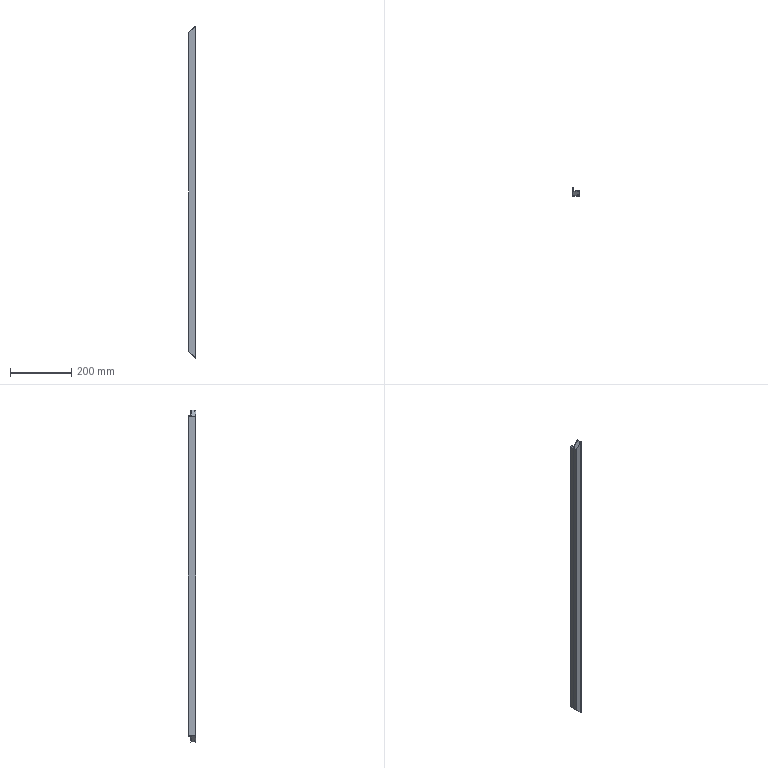Part | SolidWorks | features ICE 2, Extrusion 1 | 1 solid | 39 faces | box 22 x 25 x 1081 mm | volume 350449 mm3 | plane 22 | cylinder 17 | commonest cylinder face diameters 0.6 x2 2 x2 3.8 x2 23.6 x2 26 x2 0.97 x1
STEP:
#1=CARTESIAN_POINT('',(27.064,65.097,1061.634));
#2=VERTEX_POINT('',#1);
#3=CARTESIAN_POINT('',(26.938,66.899,1061.509));
#4=VERTEX_POINT('',#3);
#5=CARTESIAN_POINT('',(27.064,65.097,1061.634));
#6=CARTESIAN_POINT('',(26.98,65.694,1061.55));
#7=CARTESIAN_POINT('',(26.938,66.296,1061.509));
#8=CARTESIAN_POINT('',(26.938,66.899,1061.509));
#9=(BOUNDED_CURVE()B_SPLINE_CURVE(3,(#5,#6,#7,#8),.UNSPECIFIED.,.F.,.F.)B_SPLINE_CURVE_WITH_KNOTS((4,4),(6.144,6.283),.UNSPECIFIED.)CURVE()GEOMETRIC_REPRESENTATION_ITEM()RATIONAL_B_SPLINE_CURVE((1.,0.9984,0.9984,1.))REPRESENTATION_ITEM(''));
#10=EDGE_CURVE('',#2,#4,#9,.T.);
#11=ORIENTED_EDGE('',*,*,#10,.T.);
#12=CARTESIAN_POINT('',(26.938,66.899,19.491));
#13=VERTEX_POINT('',#12);
#14=CARTESIAN_POINT('',(26.938,66.899,1081.));
#15=DIRECTION('',(0.,0.,-1.));
#16=VECTOR('',#15,1000.);
#17=LINE('',#14,#16);
#18=EDGE_CURVE('',#4,#13,#17,.T.);
#19=ORIENTED_EDGE('',*,*,#18,.T.);
#20=CARTESIAN_POINT('',(27.064,65.097,19.366));
#21=VERTEX_POINT('',#20);
#22=CARTESIAN_POINT('',(27.064,65.097,19.366));
#23=CARTESIAN_POINT('',(26.98,65.694,19.45));
#24=CARTESIAN_POINT('',(26.938,66.296,19.491));
#25=CARTESIAN_POINT('',(26.938,66.899,19.491));
#26=(BOUNDED_CURVE()B_SPLINE_CURVE(3,(#22,#23,#24,#25),.UNSPECIFIED.,.F.,.T.)B_SPLINE_CURVE_WITH_KNOTS((4,4),(3.002,3.142),.UNSPECIFIED.)CURVE()GEOMETRIC_REPRESENTATION_ITEM()RATIONAL_B_SPLINE_CURVE((1.,0.9984,0.9984,1.))REPRESENTATION_ITEM(''));
#27=EDGE_CURVE('',#21,#13,#26,.T.);
#28=ORIENTED_EDGE('',*,*,#27,.F.);
#29=CARTESIAN_POINT('',(27.064,65.097,1081.));
#30=DIRECTION('',(0.,0.,-1.));
#31=VECTOR('',#30,1000.);
#32=LINE('',#29,#31);
#33=EDGE_CURVE('',#2,#21,#32,.T.);
#34=ORIENTED_EDGE('',*,*,#33,.F.);
#35=EDGE_LOOP('',(#11,#19,#28,#34));
#36=FACE_OUTER_BOUND('',#35,.T.);
#37=CARTESIAN_POINT('',(39.938,66.899,1081.));
#38=DIRECTION('',(0.,0.,-1.));
#39=DIRECTION('',(-1.,0.,0.));
#40=AXIS2_PLACEMENT_3D('',#37,#38,#39);
#41=CYLINDRICAL_SURFACE('',#40,13.);
#42=ADVANCED_FACE('',(#36),#41,.T.);
#43=CARTESIAN_POINT('',(28.252,68.536,1062.823));
#44=VERTEX_POINT('',#43);
#45=CARTESIAN_POINT('',(28.138,66.899,1062.709));
#46=VERTEX_POINT('',#45);
#47=CARTESIAN_POINT('',(28.252,68.536,1062.823));
#48=CARTESIAN_POINT('',(28.176,67.993,1062.747));
#49=CARTESIAN_POINT('',(28.138,67.447,1062.709));
#50=CARTESIAN_POINT('',(28.138,66.899,1062.709));
#51=(BOUNDED_CURVE()B_SPLINE_CURVE(3,(#47,#48,#49,#50),.UNSPECIFIED.,.F.,.F.)B_SPLINE_CURVE_WITH_KNOTS((4,4),(6.144,6.283),.UNSPECIFIED.)CURVE()GEOMETRIC_REPRESENTATION_ITEM()RATIONAL_B_SPLINE_CURVE((1.,0.9984,0.9984,1.))REPRESENTATION_ITEM(''));
#52=EDGE_CURVE('',#44,#46,#51,.T.);
#53=ORIENTED_EDGE('',*,*,#52,.T.);
#54=CARTESIAN_POINT('',(28.138,66.899,18.291));
#55=VERTEX_POINT('',#54);
#56=CARTESIAN_POINT('',(28.138,66.899,1081.));
#57=DIRECTION('',(0.,0.,-1.));
#58=VECTOR('',#57,1000.);
#59=LINE('',#56,#58);
#60=EDGE_CURVE('',#46,#55,#59,.T.);
#61=ORIENTED_EDGE('',*,*,#60,.T.);
#62=CARTESIAN_POINT('',(28.252,68.536,18.177));
#63=VERTEX_POINT('',#62);
#64=CARTESIAN_POINT('',(28.252,68.536,18.177));
#65=CARTESIAN_POINT('',(28.176,67.993,18.253));
#66=CARTESIAN_POINT('',(28.138,67.447,18.291));
#67=CARTESIAN_POINT('',(28.138,66.899,18.291));
#68=(BOUNDED_CURVE()B_SPLINE_CURVE(3,(#64,#65,#66,#67),.UNSPECIFIED.,.F.,.F.)B_SPLINE_CURVE_WITH_KNOTS((4,4),(3.002,3.142),.UNSPECIFIED.)CURVE()GEOMETRIC_REPRESENTATION_ITEM()RATIONAL_B_SPLINE_CURVE((1.,0.9984,0.9984,1.))REPRESENTATION_ITEM(''));
#69=EDGE_CURVE('',#63,#55,#68,.T.);
#70=ORIENTED_EDGE('',*,*,#69,.F.);
#71=CARTESIAN_POINT('',(28.252,68.536,1081.));
#72=DIRECTION('',(0.,0.,-1.));
#73=VECTOR('',#72,1000.);
#74=LINE('',#71,#73);
#75=EDGE_CURVE('',#44,#63,#74,.T.);
#76=ORIENTED_EDGE('',*,*,#75,.F.);
#77=EDGE_LOOP('',(#53,#61,#70,#76));
#78=FACE_OUTER_BOUND('',#77,.T.);
#79=CARTESIAN_POINT('',(39.938,66.899,1081.));
#80=DIRECTION('',(0.,0.,-1.));
#81=DIRECTION('',(-1.,0.,0.));
#82=AXIS2_PLACEMENT_3D('',#79,#80,#81);
#83=CYLINDRICAL_SURFACE('',#82,11.8);
#84=ADVANCED_FACE('',(#78),#83,.F.);
#85=CARTESIAN_POINT('',(44.608,52.847,1079.178));
#86=VERTEX_POINT('',#85);
#87=CARTESIAN_POINT('',(41.6,51.304,1076.17));
#88=VERTEX_POINT('',#87);
#89=CARTESIAN_POINT('',(44.608,52.847,1079.178));
#90=CARTESIAN_POINT('',(43.172,53.878,1077.743));
#91=CARTESIAN_POINT('',(41.6,53.071,1076.17));
#92=CARTESIAN_POINT('',(41.6,51.304,1076.17));
#93=(BOUNDED_CURVE()B_SPLINE_CURVE(3,(#89,#90,#91,#92),.UNSPECIFIED.,.F.,.F.)B_SPLINE_CURVE_WITH_KNOTS((4,4),(4.09,6.283),.UNSPECIFIED.)CURVE()GEOMETRIC_REPRESENTATION_ITEM()RATIONAL_B_SPLINE_CURVE((1.,0.6376,0.6376,1.))REPRESENTATION_ITEM(''));
#94=EDGE_CURVE('',#86,#88,#93,.T.);
#95=ORIENTED_EDGE('',*,*,#94,.T.);
#96=CARTESIAN_POINT('',(41.6,51.304,4.83));
#97=VERTEX_POINT('',#96);
#98=CARTESIAN_POINT('',(41.6,51.304,1081.));
#99=DIRECTION('',(0.,0.,-1.));
#100=VECTOR('',#99,1000.);
#101=LINE('',#98,#100);
#102=EDGE_CURVE('',#88,#97,#101,.T.);
#103=ORIENTED_EDGE('',*,*,#102,.T.);
#104=CARTESIAN_POINT('',(44.608,52.847,1.822));
#105=VERTEX_POINT('',#104);
#106=CARTESIAN_POINT('',(44.608,52.847,1.822));
#107=CARTESIAN_POINT('',(43.172,53.878,3.257));
#108=CARTESIAN_POINT('',(41.6,53.071,4.83));
#109=CARTESIAN_POINT('',(41.6,51.304,4.83));
#110=(BOUNDED_CURVE()B_SPLINE_CURVE(3,(#106,#107,#108,#109),.UNSPECIFIED.,.F.,.F.)B_SPLINE_CURVE_WITH_KNOTS((4,4),(0.948,3.142),.UNSPECIFIED.)CURVE()GEOMETRIC_REPRESENTATION_ITEM()RATIONAL_B_SPLINE_CURVE((1.,0.6376,0.6376,1.))REPRESENTATION_ITEM(''));
#111=EDGE_CURVE('',#105,#97,#110,.T.);
#112=ORIENTED_EDGE('',*,*,#111,.F.);
#113=CARTESIAN_POINT('',(44.608,52.847,1081.));
#114=DIRECTION('',(0.,0.,-1.));
#115=VECTOR('',#114,1000.);
#116=LINE('',#113,#115);
#117=EDGE_CURVE('',#86,#105,#116,.T.);
#118=ORIENTED_EDGE('',*,*,#117,.F.);
#119=EDGE_LOOP('',(#95,#103,#112,#118));
#120=FACE_OUTER_BOUND('',#119,.T.);
#121=CARTESIAN_POINT('',(43.5,51.304,1081.));
#122=DIRECTION('',(0.,0.,-1.));
#123=DIRECTION('',(-1.,0.,0.));
#124=AXIS2_PLACEMENT_3D('',#121,#122,#123);
#125=CYLINDRICAL_SURFACE('',#124,1.9);
#126=ADVANCED_FACE('',(#120),#125,.F.);
#127=CARTESIAN_POINT('',(45.44,49.348,1080.01));
#128=VERTEX_POINT('',#127);
#129=CARTESIAN_POINT('',(45.43,49.204,1080.));
#130=VERTEX_POINT('',#129);
#131=CARTESIAN_POINT('',(45.44,49.348,1080.01));
#132=CARTESIAN_POINT('',(45.433,49.3,1080.003));
#133=CARTESIAN_POINT('',(45.43,49.252,1080.));
#134=CARTESIAN_POINT('',(45.43,49.204,1080.));
#135=(BOUNDED_CURVE()B_SPLINE_CURVE(3,(#131,#132,#133,#134),.UNSPECIFIED.,.F.,.F.)B_SPLINE_CURVE_WITH_KNOTS((4,4),(6.138,6.283),.UNSPECIFIED.)CURVE()GEOMETRIC_REPRESENTATION_ITEM()RATIONAL_B_SPLINE_CURVE((1.,0.9983,0.9983,1.))REPRESENTATION_ITEM(''));
#136=EDGE_CURVE('',#128,#130,#135,.T.);
#137=ORIENTED_EDGE('',*,*,#136,.T.);
#138=CARTESIAN_POINT('',(45.43,49.204,1.));
#139=VERTEX_POINT('',#138);
#140=CARTESIAN_POINT('',(45.43,49.204,1081.));
#141=DIRECTION('',(0.,0.,-1.));
#142=VECTOR('',#141,1000.);
#143=LINE('',#140,#142);
#144=EDGE_CURVE('',#130,#139,#143,.T.);
#145=ORIENTED_EDGE('',*,*,#144,.T.);
#146=CARTESIAN_POINT('',(45.44,49.348,0.9896));
#147=VERTEX_POINT('',#146);
#148=CARTESIAN_POINT('',(45.44,49.348,0.9896));
#149=CARTESIAN_POINT('',(45.433,49.3,0.9965));
#150=CARTESIAN_POINT('',(45.43,49.252,1.));
#151=CARTESIAN_POINT('',(45.43,49.204,1.));
#152=(BOUNDED_CURVE()B_SPLINE_CURVE(3,(#148,#149,#150,#151),.UNSPECIFIED.,.F.,.F.)B_SPLINE_CURVE_WITH_KNOTS((4,4),(2.997,3.142),.UNSPECIFIED.)CURVE()GEOMETRIC_REPRESENTATION_ITEM()RATIONAL_B_SPLINE_CURVE((1.,0.9983,0.9983,1.))REPRESENTATION_ITEM(''));
#153=EDGE_CURVE('',#147,#139,#152,.T.);
#154=ORIENTED_EDGE('',*,*,#153,.F.);
#155=CARTESIAN_POINT('',(45.44,49.348,1081.));
#156=DIRECTION('',(0.,0.,-1.));
#157=VECTOR('',#156,1000.);
#158=LINE('',#155,#157);
#159=EDGE_CURVE('',#128,#147,#158,.T.);
#160=ORIENTED_EDGE('',*,*,#159,.F.);
#161=EDGE_LOOP('',(#137,#145,#154,#160));
#162=FACE_OUTER_BOUND('',#161,.T.);
#163=CARTESIAN_POINT('',(46.43,49.204,1081.));
#164=DIRECTION('',(0.,0.,-1.));
#165=DIRECTION('',(-1.,0.,0.));
#166=AXIS2_PLACEMENT_3D('',#163,#164,#165);
#167=CYLINDRICAL_SURFACE('',#166,1.);
#168=ADVANCED_FACE('',(#162),#167,.F.);
#169=CARTESIAN_POINT('',(24.43,48.204,1059.));
#170=VERTEX_POINT('',#169);
#171=CARTESIAN_POINT('',(24.43,48.204,22.));
#172=VERTEX_POINT('',#171);
#173=CARTESIAN_POINT('',(24.43,48.204,1081.));
#174=DIRECTION('',(0.,0.,-1.));
#175=VECTOR('',#174,1000.);
#176=LINE('',#173,#175);
#177=EDGE_CURVE('',#170,#172,#176,.T.);
#178=ORIENTED_EDGE('',*,*,#177,.F.);
#179=CARTESIAN_POINT('',(24.43,73.204,1059.));
#180=VERTEX_POINT('',#179);
#181=CARTESIAN_POINT('',(24.43,78.204,1059.));
#182=DIRECTION('',(0.,-1.,0.));
#183=VECTOR('',#182,1000.);
#184=LINE('',#181,#183);
#185=EDGE_CURVE('',#180,#170,#184,.T.);
#186=ORIENTED_EDGE('',*,*,#185,.F.);
#187=CARTESIAN_POINT('',(24.43,73.204,22.));
#188=VERTEX_POINT('',#187);
#189=CARTESIAN_POINT('',(24.43,73.204,1081.));
#190=DIRECTION('',(0.,0.,-1.));
#191=VECTOR('',#190,1000.);
#192=LINE('',#189,#191);
#193=EDGE_CURVE('',#180,#188,#192,.T.);
#194=ORIENTED_EDGE('',*,*,#193,.T.);
#195=CARTESIAN_POINT('',(24.43,-1303.688,22.));
#196=DIRECTION('',(0.,1.,0.));
#197=VECTOR('',#196,1000.);
#198=LINE('',#195,#197);
#199=EDGE_CURVE('',#172,#188,#198,.T.);
#200=ORIENTED_EDGE('',*,*,#199,.F.);
#201=EDGE_LOOP('',(#178,#186,#194,#200));
#202=FACE_OUTER_BOUND('',#201,.T.);
#203=CARTESIAN_POINT('',(24.43,48.204,1081.));
#204=DIRECTION('',(1.,0.,0.));
#205=DIRECTION('',(0.,0.,-1.));
#206=AXIS2_PLACEMENT_3D('',#203,#204,#205);
#207=PLANE('',#206);
#208=ADVANCED_FACE('',(#202),#207,.F.);
#209=CARTESIAN_POINT('',(46.43,48.204,1081.));
#210=VERTEX_POINT('',#209);
#211=CARTESIAN_POINT('',(46.43,48.204,0.));
#212=VERTEX_POINT('',#211);
#213=CARTESIAN_POINT('',(46.43,48.204,1081.));
#214=DIRECTION('',(0.,0.,-1.));
#215=VECTOR('',#214,1000.);
#216=LINE('',#213,#215);
#217=EDGE_CURVE('',#210,#212,#216,.T.);
#218=ORIENTED_EDGE('',*,*,#217,.F.);
#219=CARTESIAN_POINT('',(46.43,48.204,1081.));
#220=DIRECTION('',(0.7071,0.,0.7071));
#221=VECTOR('',#220,1000.);
#222=LINE('',#219,#221);
#223=EDGE_CURVE('',#170,#210,#222,.T.);
#224=ORIENTED_EDGE('',*,*,#223,.F.);
#225=ORIENTED_EDGE('',*,*,#177,.T.);
#226=CARTESIAN_POINT('',(-505.07,48.204,551.5));
#227=DIRECTION('',(-0.7071,0.,0.7071));
#228=VECTOR('',#227,1000.);
#229=LINE('',#226,#228);
#230=EDGE_CURVE('',#212,#172,#229,.T.);
#231=ORIENTED_EDGE('',*,*,#230,.F.);
#232=EDGE_LOOP('',(#218,#224,#225,#231));
#233=FACE_OUTER_BOUND('',#232,.T.);
#234=CARTESIAN_POINT('',(24.43,48.204,1081.));
#235=DIRECTION('',(0.,1.,0.));
#236=DIRECTION('',(0.,0.,1.));
#237=AXIS2_PLACEMENT_3D('',#234,#235,#236);
#238=PLANE('',#237);
#239=ADVANCED_FACE('',(#233),#238,.F.);
#240=ORIENTED_EDGE('',*,*,#144,.F.);
#241=CARTESIAN_POINT('',(45.43,49.204,1080.));
#242=CARTESIAN_POINT('',(45.43,48.618,1080.));
#243=CARTESIAN_POINT('',(45.844,48.204,1080.414));
#244=CARTESIAN_POINT('',(46.43,48.204,1081.));
#245=(BOUNDED_CURVE()B_SPLINE_CURVE(3,(#241,#242,#243,#244),.UNSPECIFIED.,.F.,.F.)B_SPLINE_CURVE_WITH_KNOTS((4,4),(0.,1.571),.UNSPECIFIED.)CURVE()GEOMETRIC_REPRESENTATION_ITEM()RATIONAL_B_SPLINE_CURVE((1.,0.8047,0.8047,1.))REPRESENTATION_ITEM(''));
#246=EDGE_CURVE('',#130,#210,#245,.T.);
#247=ORIENTED_EDGE('',*,*,#246,.T.);
#248=ORIENTED_EDGE('',*,*,#217,.T.);
#249=CARTESIAN_POINT('',(45.43,49.204,1.));
#250=CARTESIAN_POINT('',(45.43,48.618,1.));
#251=CARTESIAN_POINT('',(45.844,48.204,0.5858));
#252=CARTESIAN_POINT('',(46.43,48.204,0.));
#253=(BOUNDED_CURVE()B_SPLINE_CURVE(3,(#249,#250,#251,#252),.UNSPECIFIED.,.F.,.F.)B_SPLINE_CURVE_WITH_KNOTS((4,4),(3.142,4.712),.UNSPECIFIED.)CURVE()GEOMETRIC_REPRESENTATION_ITEM()RATIONAL_B_SPLINE_CURVE((1.,0.8047,0.8047,1.))REPRESENTATION_ITEM(''));
#254=EDGE_CURVE('',#139,#212,#253,.T.);
#255=ORIENTED_EDGE('',*,*,#254,.F.);
#256=EDGE_LOOP('',(#240,#247,#248,#255));
#257=FACE_OUTER_BOUND('',#256,.T.);
#258=CARTESIAN_POINT('',(46.43,49.204,1081.));
#259=DIRECTION('',(0.,0.,-1.));
#260=DIRECTION('',(-1.,0.,0.));
#261=AXIS2_PLACEMENT_3D('',#258,#259,#260);
#262=CYLINDRICAL_SURFACE('',#261,1.);
#263=ADVANCED_FACE('',(#257),#262,.F.);
#264=CARTESIAN_POINT('',(44.663,49.801,1079.233));
#265=VERTEX_POINT('',#264);
#266=CARTESIAN_POINT('',(44.663,49.801,1.767));
#267=VERTEX_POINT('',#266);
#268=CARTESIAN_POINT('',(44.663,49.801,1081.));
#269=DIRECTION('',(0.,0.,-1.));
#270=VECTOR('',#269,1000.);
#271=LINE('',#268,#270);
#272=EDGE_CURVE('',#265,#267,#271,.T.);
#273=ORIENTED_EDGE('',*,*,#272,.F.);
#274=CARTESIAN_POINT('',(44.663,49.801,1079.233));
#275=CARTESIAN_POINT('',(45.07,50.116,1079.64));
#276=CARTESIAN_POINT('',(45.514,49.857,1080.085));
#277=CARTESIAN_POINT('',(45.44,49.348,1080.01));
#278=(BOUNDED_CURVE()B_SPLINE_CURVE(3,(#274,#275,#276,#277),.UNSPECIFIED.,.F.,.F.)B_SPLINE_CURVE_WITH_KNOTS((4,4),(0.9119,3.286),.UNSPECIFIED.)CURVE()GEOMETRIC_REPRESENTATION_ITEM()RATIONAL_B_SPLINE_CURVE((1.,0.5828,0.5828,1.))REPRESENTATION_ITEM(''));
#279=EDGE_CURVE('',#265,#128,#278,.T.);
#280=ORIENTED_EDGE('',*,*,#279,.T.);
#281=ORIENTED_EDGE('',*,*,#159,.T.);
#282=CARTESIAN_POINT('',(44.663,49.801,1.767));
#283=CARTESIAN_POINT('',(45.07,50.116,1.36));
#284=CARTESIAN_POINT('',(45.514,49.857,0.9153));
#285=CARTESIAN_POINT('',(45.44,49.348,0.9896));
#286=(BOUNDED_CURVE()B_SPLINE_CURVE(3,(#282,#283,#284,#285),.UNSPECIFIED.,.F.,.F.)B_SPLINE_CURVE_WITH_KNOTS((4,4),(4.053,6.428),.UNSPECIFIED.)CURVE()GEOMETRIC_REPRESENTATION_ITEM()RATIONAL_B_SPLINE_CURVE((1.,0.5828,0.5828,1.))REPRESENTATION_ITEM(''));
#287=EDGE_CURVE('',#267,#147,#286,.T.);
#288=ORIENTED_EDGE('',*,*,#287,.F.);
#289=EDGE_LOOP('',(#273,#280,#281,#288));
#290=FACE_OUTER_BOUND('',#289,.T.);
#291=CARTESIAN_POINT('',(44.96,49.418,1081.));
#292=DIRECTION('',(0.,0.,-1.));
#293=DIRECTION('',(-1.,0.,0.));
#294=AXIS2_PLACEMENT_3D('',#291,#292,#293);
#295=CYLINDRICAL_SURFACE('',#294,0.4852);
#296=ADVANCED_FACE('',(#290),#295,.T.);
#297=ORIENTED_EDGE('',*,*,#102,.F.);
#298=CARTESIAN_POINT('',(41.6,51.304,1076.17));
#299=CARTESIAN_POINT('',(41.6,49.489,1076.17));
#300=CARTESIAN_POINT('',(43.228,48.691,1077.799));
#301=CARTESIAN_POINT('',(44.663,49.801,1079.233));
#302=(BOUNDED_CURVE()B_SPLINE_CURVE(3,(#298,#299,#300,#301),.UNSPECIFIED.,.F.,.T.)B_SPLINE_CURVE_WITH_KNOTS((4,4),(0.,2.23),.UNSPECIFIED.)CURVE()GEOMETRIC_REPRESENTATION_ITEM()RATIONAL_B_SPLINE_CURVE((1.,0.6269,0.6269,1.))REPRESENTATION_ITEM(''));
#303=EDGE_CURVE('',#88,#265,#302,.T.);
#304=ORIENTED_EDGE('',*,*,#303,.T.);
#305=ORIENTED_EDGE('',*,*,#272,.T.);
#306=CARTESIAN_POINT('',(41.6,51.304,4.83));
#307=CARTESIAN_POINT('',(41.6,49.489,4.83));
#308=CARTESIAN_POINT('',(43.228,48.691,3.201));
#309=CARTESIAN_POINT('',(44.663,49.801,1.767));
#310=(BOUNDED_CURVE()B_SPLINE_CURVE(3,(#306,#307,#308,#309),.UNSPECIFIED.,.F.,.T.)B_SPLINE_CURVE_WITH_KNOTS((4,4),(3.142,5.371),.UNSPECIFIED.)CURVE()GEOMETRIC_REPRESENTATION_ITEM()RATIONAL_B_SPLINE_CURVE((1.,0.6269,0.6269,1.))REPRESENTATION_ITEM(''));
#311=EDGE_CURVE('',#97,#267,#310,.T.);
#312=ORIENTED_EDGE('',*,*,#311,.F.);
#313=EDGE_LOOP('',(#297,#304,#305,#312));
#314=FACE_OUTER_BOUND('',#313,.T.);
#315=CARTESIAN_POINT('',(43.5,51.304,1081.));
#316=DIRECTION('',(0.,0.,-1.));
#317=DIRECTION('',(-1.,0.,0.));
#318=AXIS2_PLACEMENT_3D('',#315,#316,#317);
#319=CYLINDRICAL_SURFACE('',#318,1.9);
#320=ADVANCED_FACE('',(#314),#319,.F.);
#321=CARTESIAN_POINT('',(45.4,53.253,1079.97));
#322=VERTEX_POINT('',#321);
#323=CARTESIAN_POINT('',(45.4,53.253,1.03));
#324=VERTEX_POINT('',#323);
#325=CARTESIAN_POINT('',(45.4,53.253,1081.));
#326=DIRECTION('',(0.,0.,-1.));
#327=VECTOR('',#326,1000.);
#328=LINE('',#325,#327);
#329=EDGE_CURVE('',#322,#324,#328,.T.);
#330=ORIENTED_EDGE('',*,*,#329,.F.);
#331=CARTESIAN_POINT('',(45.4,53.253,1079.97));
#332=CARTESIAN_POINT('',(45.4,52.788,1079.97));
#333=CARTESIAN_POINT('',(44.986,52.575,1079.556));
#334=CARTESIAN_POINT('',(44.608,52.847,1079.178));
#335=(BOUNDED_CURVE()B_SPLINE_CURVE(3,(#331,#332,#333,#334),.UNSPECIFIED.,.F.,.F.)B_SPLINE_CURVE_WITH_KNOTS((4,4),(3.142,5.335),.UNSPECIFIED.)CURVE()GEOMETRIC_REPRESENTATION_ITEM()RATIONAL_B_SPLINE_CURVE((1.,0.6376,0.6376,1.))REPRESENTATION_ITEM(''));
#336=EDGE_CURVE('',#322,#86,#335,.T.);
#337=ORIENTED_EDGE('',*,*,#336,.T.);
#338=ORIENTED_EDGE('',*,*,#117,.T.);
#339=CARTESIAN_POINT('',(45.4,53.253,1.03));
#340=CARTESIAN_POINT('',(45.4,52.788,1.03));
#341=CARTESIAN_POINT('',(44.986,52.575,1.444));
#342=CARTESIAN_POINT('',(44.608,52.847,1.822));
#343=(BOUNDED_CURVE()B_SPLINE_CURVE(3,(#339,#340,#341,#342),.UNSPECIFIED.,.F.,.F.)B_SPLINE_CURVE_WITH_KNOTS((4,4),(0.,2.194),.UNSPECIFIED.)CURVE()GEOMETRIC_REPRESENTATION_ITEM()RATIONAL_B_SPLINE_CURVE((1.,0.6376,0.6376,1.))REPRESENTATION_ITEM(''));
#344=EDGE_CURVE('',#324,#105,#343,.T.);
#345=ORIENTED_EDGE('',*,*,#344,.F.);
#346=EDGE_LOOP('',(#330,#337,#338,#345));
#347=FACE_OUTER_BOUND('',#346,.T.);
#348=CARTESIAN_POINT('',(44.9,53.253,1081.));
#349=DIRECTION('',(0.,0.,-1.));
#350=DIRECTION('',(-1.,0.,0.));
#351=AXIS2_PLACEMENT_3D('',#348,#349,#350);
#352=CYLINDRICAL_SURFACE('',#351,0.5);
#353=ADVANCED_FACE('',(#347),#352,.T.);
#354=CARTESIAN_POINT('',(45.4,58.567,1079.97));
#355=VERTEX_POINT('',#354);
#356=CARTESIAN_POINT('',(45.4,58.567,1.03));
#357=VERTEX_POINT('',#356);
#358=CARTESIAN_POINT('',(45.4,58.567,1081.));
#359=DIRECTION('',(0.,0.,-1.));
#360=VECTOR('',#359,1000.);
#361=LINE('',#358,#360);
#362=EDGE_CURVE('',#355,#357,#361,.T.);
#363=ORIENTED_EDGE('',*,*,#362,.F.);
#364=CARTESIAN_POINT('',(45.4,58.567,1079.97));
#365=DIRECTION('',(0.,-1.,0.));
#366=VECTOR('',#365,1000.);
#367=LINE('',#364,#366);
#368=EDGE_CURVE('',#355,#322,#367,.T.);
#369=ORIENTED_EDGE('',*,*,#368,.T.);
#370=ORIENTED_EDGE('',*,*,#329,.T.);
#371=CARTESIAN_POINT('',(45.4,58.567,1.03));
#372=DIRECTION('',(0.,-1.,0.));
#373=VECTOR('',#372,1000.);
#374=LINE('',#371,#373);
#375=EDGE_CURVE('',#357,#324,#374,.T.);
#376=ORIENTED_EDGE('',*,*,#375,.F.);
#377=EDGE_LOOP('',(#363,#369,#370,#376));
#378=FACE_OUTER_BOUND('',#377,.T.);
#379=CARTESIAN_POINT('',(45.4,58.567,1081.));
#380=DIRECTION('',(-1.,0.,0.));
#381=DIRECTION('',(0.,0.,1.));
#382=AXIS2_PLACEMENT_3D('',#379,#380,#381);
#383=PLANE('',#382);
#384=ADVANCED_FACE('',(#378),#383,.F.);
#385=CARTESIAN_POINT('',(41.4,62.567,1075.97));
#386=VERTEX_POINT('',#385);
#387=CARTESIAN_POINT('',(41.4,62.567,5.03));
#388=VERTEX_POINT('',#387);
#389=CARTESIAN_POINT('',(41.4,62.567,1081.));
#390=DIRECTION('',(0.,0.,-1.));
#391=VECTOR('',#390,1000.);
#392=LINE('',#389,#391);
#393=EDGE_CURVE('',#386,#388,#392,.T.);
#394=ORIENTED_EDGE('',*,*,#393,.F.);
#395=CARTESIAN_POINT('',(41.4,62.567,1075.97));
#396=CARTESIAN_POINT('',(43.743,62.567,1078.313));
#397=CARTESIAN_POINT('',(45.4,60.91,1079.97));
#398=CARTESIAN_POINT('',(45.4,58.567,1079.97));
#399=(BOUNDED_CURVE()B_SPLINE_CURVE(3,(#395,#396,#397,#398),.UNSPECIFIED.,.F.,.F.)B_SPLINE_CURVE_WITH_KNOTS((4,4),(1.571,3.142),.UNSPECIFIED.)CURVE()GEOMETRIC_REPRESENTATION_ITEM()RATIONAL_B_SPLINE_CURVE((1.,0.8047,0.8047,1.))REPRESENTATION_ITEM(''));
#400=EDGE_CURVE('',#386,#355,#399,.T.);
#401=ORIENTED_EDGE('',*,*,#400,.T.);
#402=ORIENTED_EDGE('',*,*,#362,.T.);
#403=CARTESIAN_POINT('',(41.4,62.567,5.03));
#404=CARTESIAN_POINT('',(43.743,62.567,2.687));
#405=CARTESIAN_POINT('',(45.4,60.91,1.03));
#406=CARTESIAN_POINT('',(45.4,58.567,1.03));
#407=(BOUNDED_CURVE()B_SPLINE_CURVE(3,(#403,#404,#405,#406),.UNSPECIFIED.,.F.,.T.)B_SPLINE_CURVE_WITH_KNOTS((4,4),(4.712,6.283),.UNSPECIFIED.)CURVE()GEOMETRIC_REPRESENTATION_ITEM()RATIONAL_B_SPLINE_CURVE((1.,0.8047,0.8047,1.))REPRESENTATION_ITEM(''));
#408=EDGE_CURVE('',#388,#357,#407,.T.);
#409=ORIENTED_EDGE('',*,*,#408,.F.);
#410=EDGE_LOOP('',(#394,#401,#402,#409));
#411=FACE_OUTER_BOUND('',#410,.T.);
#412=CARTESIAN_POINT('',(41.4,58.567,1081.));
#413=DIRECTION('',(0.,0.,-1.));
#414=DIRECTION('',(-1.,0.,0.));
#415=AXIS2_PLACEMENT_3D('',#412,#413,#414);
#416=CYLINDRICAL_SURFACE('',#415,4.);
#417=ADVANCED_FACE('',(#411),#416,.T.);
#418=CARTESIAN_POINT('',(35.32,62.567,1069.89));
#419=VERTEX_POINT('',#418);
#420=CARTESIAN_POINT('',(35.32,62.567,11.11));
#421=VERTEX_POINT('',#420);
#422=CARTESIAN_POINT('',(35.32,62.567,1081.));
#423=DIRECTION('',(0.,0.,-1.));
#424=VECTOR('',#423,1000.);
#425=LINE('',#422,#424);
#426=EDGE_CURVE('',#419,#421,#425,.T.);
#427=ORIENTED_EDGE('',*,*,#426,.F.);
#428=CARTESIAN_POINT('',(40.875,62.567,1075.445));
#429=DIRECTION('',(0.7071,0.,0.7071));
#430=VECTOR('',#429,1000.);
#431=LINE('',#428,#430);
#432=EDGE_CURVE('',#419,#386,#431,.T.);
#433=ORIENTED_EDGE('',*,*,#432,.T.);
#434=ORIENTED_EDGE('',*,*,#393,.T.);
#435=CARTESIAN_POINT('',(-499.625,62.567,546.055));
#436=DIRECTION('',(0.7071,0.,-0.7071));
#437=VECTOR('',#436,1000.);
#438=LINE('',#435,#437);
#439=EDGE_CURVE('',#421,#388,#438,.T.);
#440=ORIENTED_EDGE('',*,*,#439,.F.);
#441=EDGE_LOOP('',(#427,#433,#434,#440));
#442=FACE_OUTER_BOUND('',#441,.T.);
#443=CARTESIAN_POINT('',(35.32,62.567,1081.));
#444=DIRECTION('',(0.,-1.,0.));
#445=DIRECTION('',(0.,0.,-1.));
#446=AXIS2_PLACEMENT_3D('',#443,#444,#445);
#447=PLANE('',#446);
#448=ADVANCED_FACE('',(#442),#447,.F.);
#449=CARTESIAN_POINT('',(35.32,63.565,1069.89));
#450=VERTEX_POINT('',#449);
#451=CARTESIAN_POINT('',(35.32,63.565,11.11));
#452=VERTEX_POINT('',#451);
#453=CARTESIAN_POINT('',(35.32,63.565,1081.));
#454=DIRECTION('',(0.,0.,-1.));
#455=VECTOR('',#454,1000.);
#456=LINE('',#453,#455);
#457=EDGE_CURVE('',#450,#452,#456,.T.);
#458=ORIENTED_EDGE('',*,*,#457,.F.);
#459=CARTESIAN_POINT('',(35.32,63.565,1069.89));
#460=DIRECTION('',(0.,-1.,0.));
#461=VECTOR('',#460,1000.);
#462=LINE('',#459,#461);
#463=EDGE_CURVE('',#450,#419,#462,.T.);
#464=ORIENTED_EDGE('',*,*,#463,.T.);
#465=ORIENTED_EDGE('',*,*,#426,.T.);
#466=CARTESIAN_POINT('',(35.32,63.565,11.11));
#467=DIRECTION('',(0.,-1.,0.));
#468=VECTOR('',#467,1000.);
#469=LINE('',#466,#468);
#470=EDGE_CURVE('',#452,#421,#469,.T.);
#471=ORIENTED_EDGE('',*,*,#470,.F.);
#472=EDGE_LOOP('',(#458,#464,#465,#471));
#473=FACE_OUTER_BOUND('',#472,.T.);
#474=CARTESIAN_POINT('',(35.32,63.565,1081.));
#475=DIRECTION('',(-1.,0.,0.));
#476=DIRECTION('',(0.,0.,1.));
#477=AXIS2_PLACEMENT_3D('',#474,#475,#476);
#478=PLANE('',#477);
#479=ADVANCED_FACE('',(#473),#478,.F.);
#480=CARTESIAN_POINT('',(37.522,63.233,1072.093));
#481=VERTEX_POINT('',#480);
#482=CARTESIAN_POINT('',(37.522,63.233,8.907));
#483=VERTEX_POINT('',#482);
#484=CARTESIAN_POINT('',(37.522,63.233,1081.));
#485=DIRECTION('',(0.,0.,-1.));
#486=VECTOR('',#485,1000.);
#487=LINE('',#484,#486);
#488=EDGE_CURVE('',#481,#483,#487,.T.);
#489=ORIENTED_EDGE('',*,*,#488,.F.);
#490=CARTESIAN_POINT('',(37.522,63.233,1072.093));
#491=CARTESIAN_POINT('',(36.804,63.437,1071.375));
#492=CARTESIAN_POINT('',(36.066,63.548,1070.636));
#493=CARTESIAN_POINT('',(35.32,63.565,1069.89));
#494=(BOUNDED_CURVE()B_SPLINE_CURVE(3,(#490,#491,#492,#493),.UNSPECIFIED.,.F.,.T.)B_SPLINE_CURVE_WITH_KNOTS((4,4),(4.436,4.69),.UNSPECIFIED.)CURVE()GEOMETRIC_REPRESENTATION_ITEM()RATIONAL_B_SPLINE_CURVE((1.,0.9946,0.9946,1.))REPRESENTATION_ITEM(''));
#495=EDGE_CURVE('',#481,#450,#494,.T.);
#496=ORIENTED_EDGE('',*,*,#495,.T.);
#497=ORIENTED_EDGE('',*,*,#457,.T.);
#498=CARTESIAN_POINT('',(37.522,63.233,8.907));
#499=CARTESIAN_POINT('',(36.804,63.437,9.625));
#500=CARTESIAN_POINT('',(36.066,63.548,10.364));
#501=CARTESIAN_POINT('',(35.32,63.565,11.11));
#502=(BOUNDED_CURVE()B_SPLINE_CURVE(3,(#498,#499,#500,#501),.UNSPECIFIED.,.F.,.T.)B_SPLINE_CURVE_WITH_KNOTS((4,4),(1.294,1.548),.UNSPECIFIED.)CURVE()GEOMETRIC_REPRESENTATION_ITEM()RATIONAL_B_SPLINE_CURVE((1.,0.9946,0.9946,1.))REPRESENTATION_ITEM(''));
#503=EDGE_CURVE('',#483,#452,#502,.T.);
#504=ORIENTED_EDGE('',*,*,#503,.F.);
#505=EDGE_LOOP('',(#489,#496,#497,#504));
#506=FACE_OUTER_BOUND('',#505,.T.);
#507=CARTESIAN_POINT('',(35.12,54.767,1081.));
#508=DIRECTION('',(0.,0.,-1.));
#509=DIRECTION('',(-1.,0.,0.));
#510=AXIS2_PLACEMENT_3D('',#507,#508,#509);
#511=CYLINDRICAL_SURFACE('',#510,8.8);
#512=ADVANCED_FACE('',(#506),#511,.F.);
#513=CARTESIAN_POINT('',(43.408,63.335,1077.978));
#514=VERTEX_POINT('',#513);
#515=CARTESIAN_POINT('',(43.408,63.335,3.022));
#516=VERTEX_POINT('',#515);
#517=CARTESIAN_POINT('',(43.408,63.335,1081.));
#518=DIRECTION('',(0.,0.,-1.));
#519=VECTOR('',#518,1000.);
#520=LINE('',#517,#519);
#521=EDGE_CURVE('',#514,#516,#520,.T.);
#522=ORIENTED_EDGE('',*,*,#521,.F.);
#523=CARTESIAN_POINT('',(43.408,63.335,1077.978));
#524=CARTESIAN_POINT('',(41.485,62.716,1076.056));
#525=CARTESIAN_POINT('',(39.466,62.681,1074.036));
#526=CARTESIAN_POINT('',(37.522,63.233,1072.093));
#527=(BOUNDED_CURVE()B_SPLINE_CURVE(3,(#523,#524,#525,#526),.UNSPECIFIED.,.F.,.F.)B_SPLINE_CURVE_WITH_KNOTS((4,4),(4.401,4.989),.UNSPECIFIED.)CURVE()GEOMETRIC_REPRESENTATION_ITEM()RATIONAL_B_SPLINE_CURVE((1.,0.9714,0.9714,1.))REPRESENTATION_ITEM(''));
#528=EDGE_CURVE('',#514,#481,#527,.T.);
#529=ORIENTED_EDGE('',*,*,#528,.T.);
#530=ORIENTED_EDGE('',*,*,#488,.T.);
#531=CARTESIAN_POINT('',(43.408,63.335,3.022));
#532=CARTESIAN_POINT('',(41.485,62.716,4.944));
#533=CARTESIAN_POINT('',(39.466,62.681,6.964));
#534=CARTESIAN_POINT('',(37.522,63.233,8.907));
#535=(BOUNDED_CURVE()B_SPLINE_CURVE(3,(#531,#532,#533,#534),.UNSPECIFIED.,.F.,.F.)B_SPLINE_CURVE_WITH_KNOTS((4,4),(1.26,1.847),.UNSPECIFIED.)CURVE()GEOMETRIC_REPRESENTATION_ITEM()RATIONAL_B_SPLINE_CURVE((1.,0.9714,0.9714,1.))REPRESENTATION_ITEM(''));
#536=EDGE_CURVE('',#516,#483,#535,.T.);
#537=ORIENTED_EDGE('',*,*,#536,.F.);
#538=EDGE_LOOP('',(#522,#529,#530,#537));
#539=FACE_OUTER_BOUND('',#538,.T.);
#540=CARTESIAN_POINT('',(40.297,73.007,1081.));
#541=DIRECTION('',(0.,0.,-1.));
#542=DIRECTION('',(-1.,0.,0.));
#543=AXIS2_PLACEMENT_3D('',#540,#541,#542);
#544=CYLINDRICAL_SURFACE('',#543,10.16);
#545=ADVANCED_FACE('',(#539),#544,.T.);
#546=CARTESIAN_POINT('',(46.43,64.307,1081.));
#547=VERTEX_POINT('',#546);
#548=CARTESIAN_POINT('',(46.43,64.307,0.));
#549=VERTEX_POINT('',#548);
#550=CARTESIAN_POINT('',(46.43,64.307,1081.));
#551=DIRECTION('',(0.,0.,-1.));
#552=VECTOR('',#551,1000.);
#553=LINE('',#550,#552);
#554=EDGE_CURVE('',#547,#549,#553,.T.);
#555=ORIENTED_EDGE('',*,*,#554,.F.);
#556=CARTESIAN_POINT('',(44.844,63.797,1079.415));
#557=DIRECTION('',(-0.6895,-0.2218,-0.6895));
#558=VECTOR('',#557,1000.);
#559=LINE('',#556,#558);
#560=EDGE_CURVE('',#547,#514,#559,.T.);
#561=ORIENTED_EDGE('',*,*,#560,.T.);
#562=ORIENTED_EDGE('',*,*,#521,.T.);
#563=CARTESIAN_POINT('',(-469.064,-101.524,515.494));
#564=DIRECTION('',(-0.6895,-0.2218,0.6895));
#565=VECTOR('',#564,1000.);
#566=LINE('',#563,#565);
#567=EDGE_CURVE('',#549,#516,#566,.T.);
#568=ORIENTED_EDGE('',*,*,#567,.F.);
#569=EDGE_LOOP('',(#555,#561,#562,#568));
#570=FACE_OUTER_BOUND('',#569,.T.);
#571=CARTESIAN_POINT('',(43.408,63.335,1081.));
#572=DIRECTION('',(-0.3062,0.952,0.));
#573=DIRECTION('',(-0.952,-0.3062,0.));
#574=AXIS2_PLACEMENT_3D('',#571,#572,#573);
#575=PLANE('',#574);
#576=ADVANCED_FACE('',(#570),#575,.F.);
#577=CARTESIAN_POINT('',(43.041,64.477,1077.611));
#578=VERTEX_POINT('',#577);
#579=CARTESIAN_POINT('',(43.041,64.477,3.389));
#580=VERTEX_POINT('',#579);
#581=CARTESIAN_POINT('',(43.041,64.477,1081.));
#582=DIRECTION('',(0.,0.,-1.));
#583=VECTOR('',#582,1000.);
#584=LINE('',#581,#583);
#585=EDGE_CURVE('',#578,#580,#584,.T.);
#586=ORIENTED_EDGE('',*,*,#585,.F.);
#587=CARTESIAN_POINT('',(46.43,65.567,1081.));
#588=VERTEX_POINT('',#587);
#589=CARTESIAN_POINT('',(44.652,64.995,1079.222));
#590=DIRECTION('',(0.6895,0.2218,0.6895));
#591=VECTOR('',#590,1000.);
#592=LINE('',#589,#591);
#593=EDGE_CURVE('',#578,#588,#592,.T.);
#594=ORIENTED_EDGE('',*,*,#593,.T.);
#595=CARTESIAN_POINT('',(46.43,65.567,0.));
#596=VERTEX_POINT('',#595);
#597=CARTESIAN_POINT('',(46.43,65.567,1081.));
#598=DIRECTION('',(0.,0.,-1.));
#599=VECTOR('',#598,1000.);
#600=LINE('',#597,#599);
#601=EDGE_CURVE('',#588,#596,#600,.T.);
#602=ORIENTED_EDGE('',*,*,#601,.T.);
#603=CARTESIAN_POINT('',(-469.257,-100.325,515.687));
#604=DIRECTION('',(0.6895,0.2218,-0.6895));
#605=VECTOR('',#604,1000.);
#606=LINE('',#603,#605);
#607=EDGE_CURVE('',#580,#596,#606,.T.);
#608=ORIENTED_EDGE('',*,*,#607,.F.);
#609=EDGE_LOOP('',(#586,#594,#602,#608));
#610=FACE_OUTER_BOUND('',#609,.T.);
#611=CARTESIAN_POINT('',(43.041,64.477,1081.));
#612=DIRECTION('',(0.3062,-0.952,0.));
#613=DIRECTION('',(0.952,0.3062,0.));
#614=AXIS2_PLACEMENT_3D('',#611,#612,#613);
#615=PLANE('',#614);
#616=ADVANCED_FACE('',(#610),#615,.F.);
#617=CARTESIAN_POINT('',(37.85,64.387,1072.42));
#618=VERTEX_POINT('',#617);
#619=CARTESIAN_POINT('',(37.85,64.387,8.58));
#620=VERTEX_POINT('',#619);
#621=CARTESIAN_POINT('',(37.85,64.387,1081.));
#622=DIRECTION('',(0.,0.,-1.));
#623=VECTOR('',#622,1000.);
#624=LINE('',#621,#623);
#625=EDGE_CURVE('',#618,#620,#624,.T.);
#626=ORIENTED_EDGE('',*,*,#625,.F.);
#627=CARTESIAN_POINT('',(37.85,64.387,1072.42));
#628=CARTESIAN_POINT('',(39.564,63.901,1074.134));
#629=CARTESIAN_POINT('',(41.345,63.932,1075.915));
#630=CARTESIAN_POINT('',(43.041,64.477,1077.611));
#631=(BOUNDED_CURVE()B_SPLINE_CURVE(3,(#627,#628,#629,#630),.UNSPECIFIED.,.F.,.F.)B_SPLINE_CURVE_WITH_KNOTS((4,4),(1.294,1.882),.UNSPECIFIED.)CURVE()GEOMETRIC_REPRESENTATION_ITEM()RATIONAL_B_SPLINE_CURVE((1.,0.9714,0.9714,1.))REPRESENTATION_ITEM(''));
#632=EDGE_CURVE('',#618,#578,#631,.T.);
#633=ORIENTED_EDGE('',*,*,#632,.T.);
#634=ORIENTED_EDGE('',*,*,#585,.T.);
#635=CARTESIAN_POINT('',(37.85,64.387,8.58));
#636=CARTESIAN_POINT('',(39.564,63.901,6.866));
#637=CARTESIAN_POINT('',(41.345,63.932,5.085));
#638=CARTESIAN_POINT('',(43.041,64.477,3.389));
#639=(BOUNDED_CURVE()B_SPLINE_CURVE(3,(#635,#636,#637,#638),.UNSPECIFIED.,.F.,.F.)B_SPLINE_CURVE_WITH_KNOTS((4,4),(4.436,5.024),.UNSPECIFIED.)CURVE()GEOMETRIC_REPRESENTATION_ITEM()RATIONAL_B_SPLINE_CURVE((1.,0.9714,0.9714,1.))REPRESENTATION_ITEM(''));
#640=EDGE_CURVE('',#620,#580,#639,.T.);
#641=ORIENTED_EDGE('',*,*,#640,.F.);
#642=EDGE_LOOP('',(#626,#633,#634,#641));
#643=FACE_OUTER_BOUND('',#642,.T.);
#644=CARTESIAN_POINT('',(40.297,73.007,1081.));
#645=DIRECTION('',(0.,0.,-1.));
#646=DIRECTION('',(-1.,0.,0.));
#647=AXIS2_PLACEMENT_3D('',#644,#645,#646);
#648=CYLINDRICAL_SURFACE('',#647,8.96);
#649=ADVANCED_FACE('',(#643),#648,.F.);
#650=CARTESIAN_POINT('',(35.12,64.767,1069.69));
#651=VERTEX_POINT('',#650);
#652=CARTESIAN_POINT('',(35.12,64.767,11.31));
#653=VERTEX_POINT('',#652);
#654=CARTESIAN_POINT('',(35.12,64.767,1081.));
#655=DIRECTION('',(0.,0.,-1.));
#656=VECTOR('',#655,1000.);
#657=LINE('',#654,#656);
#658=EDGE_CURVE('',#651,#653,#657,.T.);
#659=ORIENTED_EDGE('',*,*,#658,.F.);
#660=CARTESIAN_POINT('',(35.12,64.767,1069.69));
#661=CARTESIAN_POINT('',(36.044,64.767,1070.615));
#662=CARTESIAN_POINT('',(36.96,64.64,1071.531));
#663=CARTESIAN_POINT('',(37.85,64.387,1072.42));
#664=(BOUNDED_CURVE()B_SPLINE_CURVE(3,(#660,#661,#662,#663),.UNSPECIFIED.,.F.,.F.)B_SPLINE_CURVE_WITH_KNOTS((4,4),(1.571,1.847),.UNSPECIFIED.)CURVE()GEOMETRIC_REPRESENTATION_ITEM()RATIONAL_B_SPLINE_CURVE((1.,0.9936,0.9936,1.))REPRESENTATION_ITEM(''));
#665=EDGE_CURVE('',#651,#618,#664,.T.);
#666=ORIENTED_EDGE('',*,*,#665,.T.);
#667=ORIENTED_EDGE('',*,*,#625,.T.);
#668=CARTESIAN_POINT('',(35.12,64.767,11.31));
#669=CARTESIAN_POINT('',(36.044,64.767,10.385));
#670=CARTESIAN_POINT('',(36.96,64.64,9.469));
#671=CARTESIAN_POINT('',(37.85,64.387,8.58));
#672=(BOUNDED_CURVE()B_SPLINE_CURVE(3,(#668,#669,#670,#671),.UNSPECIFIED.,.F.,.T.)B_SPLINE_CURVE_WITH_KNOTS((4,4),(4.712,4.989),.UNSPECIFIED.)CURVE()GEOMETRIC_REPRESENTATION_ITEM()RATIONAL_B_SPLINE_CURVE((1.,0.9936,0.9936,1.))REPRESENTATION_ITEM(''));
#673=EDGE_CURVE('',#653,#620,#672,.T.);
#674=ORIENTED_EDGE('',*,*,#673,.F.);
#675=EDGE_LOOP('',(#659,#666,#667,#674));
#676=FACE_OUTER_BOUND('',#675,.T.);
#677=CARTESIAN_POINT('',(35.12,54.767,1081.));
#678=DIRECTION('',(0.,0.,-1.));
#679=DIRECTION('',(-1.,0.,0.));
#680=AXIS2_PLACEMENT_3D('',#677,#678,#679);
#681=CYLINDRICAL_SURFACE('',#680,10.);
#682=ADVANCED_FACE('',(#676),#681,.T.);
#683=CARTESIAN_POINT('',(34.12,64.767,1068.69));
#684=VERTEX_POINT('',#683);
#685=CARTESIAN_POINT('',(34.12,64.767,12.31));
#686=VERTEX_POINT('',#685);
#687=CARTESIAN_POINT('',(34.12,64.767,1081.));
#688=DIRECTION('',(0.,0.,-1.));
#689=VECTOR('',#688,1000.);
#690=LINE('',#687,#689);
#691=EDGE_CURVE('',#684,#686,#690,.T.);
#692=ORIENTED_EDGE('',*,*,#691,.F.);
#693=CARTESIAN_POINT('',(40.275,64.767,1074.845));
#694=DIRECTION('',(0.7071,0.,0.7071));
#695=VECTOR('',#694,1000.);
#696=LINE('',#693,#695);
#697=EDGE_CURVE('',#684,#651,#696,.T.);
#698=ORIENTED_EDGE('',*,*,#697,.T.);
#699=ORIENTED_EDGE('',*,*,#658,.T.);
#700=CARTESIAN_POINT('',(-500.225,64.767,546.655));
#701=DIRECTION('',(0.7071,0.,-0.7071));
#702=VECTOR('',#701,1000.);
#703=LINE('',#700,#702);
#704=EDGE_CURVE('',#686,#653,#703,.T.);
#705=ORIENTED_EDGE('',*,*,#704,.F.);
#706=EDGE_LOOP('',(#692,#698,#699,#705));
#707=FACE_OUTER_BOUND('',#706,.T.);
#708=CARTESIAN_POINT('',(34.12,64.767,1081.));
#709=DIRECTION('',(0.,-1.,0.));
#710=DIRECTION('',(0.,0.,-1.));
#711=AXIS2_PLACEMENT_3D('',#708,#709,#710);
#712=PLANE('',#711);
#713=ADVANCED_FACE('',(#707),#712,.F.);
#714=CARTESIAN_POINT('',(34.12,62.567,1068.69));
#715=VERTEX_POINT('',#714);
#716=CARTESIAN_POINT('',(34.12,62.567,12.31));
#717=VERTEX_POINT('',#716);
#718=CARTESIAN_POINT('',(34.12,62.567,1081.));
#719=DIRECTION('',(0.,0.,-1.));
#720=VECTOR('',#719,1000.);
#721=LINE('',#718,#720);
#722=EDGE_CURVE('',#715,#717,#721,.T.);
#723=ORIENTED_EDGE('',*,*,#722,.F.);
#724=CARTESIAN_POINT('',(34.12,62.567,1068.69));
#725=DIRECTION('',(0.,1.,0.));
#726=VECTOR('',#725,1000.);
#727=LINE('',#724,#726);
#728=EDGE_CURVE('',#715,#684,#727,.T.);
#729=ORIENTED_EDGE('',*,*,#728,.T.);
#730=ORIENTED_EDGE('',*,*,#691,.T.);
#731=CARTESIAN_POINT('',(34.12,62.567,12.31));
#732=DIRECTION('',(0.,1.,0.));
#733=VECTOR('',#732,1000.);
#734=LINE('',#731,#733);
#735=EDGE_CURVE('',#717,#686,#734,.T.);
#736=ORIENTED_EDGE('',*,*,#735,.F.);
#737=EDGE_LOOP('',(#723,#729,#730,#736));
#738=FACE_OUTER_BOUND('',#737,.T.);
#739=CARTESIAN_POINT('',(34.12,62.567,1081.));
#740=DIRECTION('',(1.,0.,0.));
#741=DIRECTION('',(0.,0.,-1.));
#742=AXIS2_PLACEMENT_3D('',#739,#740,#741);
#743=PLANE('',#742);
#744=ADVANCED_FACE('',(#738),#743,.F.);
#745=CARTESIAN_POINT('',(28.63,62.567,1063.2));
#746=VERTEX_POINT('',#745);
#747=CARTESIAN_POINT('',(28.63,62.567,17.8));
#748=VERTEX_POINT('',#747);
#749=CARTESIAN_POINT('',(28.63,62.567,1081.));
#750=DIRECTION('',(0.,0.,-1.));
#751=VECTOR('',#750,1000.);
#752=LINE('',#749,#751);
#753=EDGE_CURVE('',#746,#748,#752,.T.);
#754=ORIENTED_EDGE('',*,*,#753,.F.);
#755=CARTESIAN_POINT('',(37.53,62.567,1072.1));
#756=DIRECTION('',(0.7071,0.,0.7071));
#757=VECTOR('',#756,1000.);
#758=LINE('',#755,#757);
#759=EDGE_CURVE('',#746,#715,#758,.T.);
#760=ORIENTED_EDGE('',*,*,#759,.T.);
#761=ORIENTED_EDGE('',*,*,#722,.T.);
#762=CARTESIAN_POINT('',(-502.97,62.567,549.4));
#763=DIRECTION('',(0.7071,0.,-0.7071));
#764=VECTOR('',#763,1000.);
#765=LINE('',#762,#764);
#766=EDGE_CURVE('',#748,#717,#765,.T.);
#767=ORIENTED_EDGE('',*,*,#766,.F.);
#768=EDGE_LOOP('',(#754,#760,#761,#767));
#769=FACE_OUTER_BOUND('',#768,.T.);
#770=CARTESIAN_POINT('',(28.63,62.567,1081.));
#771=DIRECTION('',(0.,-1.,0.));
#772=DIRECTION('',(0.,0.,-1.));
#773=AXIS2_PLACEMENT_3D('',#770,#771,#772);
#774=PLANE('',#773);
#775=ADVANCED_FACE('',(#769),#774,.F.);
#776=CARTESIAN_POINT('',(28.252,65.263,1062.823));
#777=VERTEX_POINT('',#776);
#778=CARTESIAN_POINT('',(28.252,65.263,18.177));
#779=VERTEX_POINT('',#778);
#780=CARTESIAN_POINT('',(28.252,65.263,1081.));
#781=DIRECTION('',(0.,0.,-1.));
#782=VECTOR('',#781,1000.);
#783=LINE('',#780,#782);
#784=EDGE_CURVE('',#777,#779,#783,.T.);
#785=ORIENTED_EDGE('',*,*,#784,.F.);
#786=CARTESIAN_POINT('',(28.595,62.815,1063.165));
#787=DIRECTION('',(0.1373,-0.981,0.1373));
#788=VECTOR('',#787,1000.);
#789=LINE('',#786,#788);
#790=EDGE_CURVE('',#777,#746,#789,.T.);
#791=ORIENTED_EDGE('',*,*,#790,.T.);
#792=ORIENTED_EDGE('',*,*,#753,.T.);
#793=CARTESIAN_POINT('',(8.207,208.446,38.223));
#794=DIRECTION('',(0.1373,-0.981,-0.1373));
#795=VECTOR('',#794,1000.);
#796=LINE('',#793,#795);
#797=EDGE_CURVE('',#779,#748,#796,.T.);
#798=ORIENTED_EDGE('',*,*,#797,.F.);
#799=EDGE_LOOP('',(#785,#791,#792,#798));
#800=FACE_OUTER_BOUND('',#799,.T.);
#801=CARTESIAN_POINT('',(28.252,65.263,1081.));
#802=DIRECTION('',(-0.9903,-0.1386,0.));
#803=DIRECTION('',(0.1386,-0.9903,0.));
#804=AXIS2_PLACEMENT_3D('',#801,#802,#803);
#805=PLANE('',#804);
#806=ADVANCED_FACE('',(#800),#805,.F.);
#807=ORIENTED_EDGE('',*,*,#60,.F.);
#808=CARTESIAN_POINT('',(28.138,66.899,1062.709));
#809=CARTESIAN_POINT('',(28.138,66.352,1062.709));
#810=CARTESIAN_POINT('',(28.176,65.806,1062.747));
#811=CARTESIAN_POINT('',(28.252,65.263,1062.823));
#812=(BOUNDED_CURVE()B_SPLINE_CURVE(3,(#808,#809,#810,#811),.UNSPECIFIED.,.F.,.F.)B_SPLINE_CURVE_WITH_KNOTS((4,4),(0.,0.1391),.UNSPECIFIED.)CURVE()GEOMETRIC_REPRESENTATION_ITEM()RATIONAL_B_SPLINE_CURVE((1.,0.9984,0.9984,1.))REPRESENTATION_ITEM(''));
#813=EDGE_CURVE('',#46,#777,#812,.T.);
#814=ORIENTED_EDGE('',*,*,#813,.T.);
#815=ORIENTED_EDGE('',*,*,#784,.T.);
#816=CARTESIAN_POINT('',(28.138,66.899,18.291));
#817=CARTESIAN_POINT('',(28.138,66.352,18.291));
#818=CARTESIAN_POINT('',(28.176,65.806,18.253));
#819=CARTESIAN_POINT('',(28.252,65.263,18.177));
#820=(BOUNDED_CURVE()B_SPLINE_CURVE(3,(#816,#817,#818,#819),.UNSPECIFIED.,.F.,.F.)B_SPLINE_CURVE_WITH_KNOTS((4,4),(3.142,3.281),.UNSPECIFIED.)CURVE()GEOMETRIC_REPRESENTATION_ITEM()RATIONAL_B_SPLINE_CURVE((1.,0.9984,0.9984,1.))REPRESENTATION_ITEM(''));
#821=EDGE_CURVE('',#55,#779,#820,.T.);
#822=ORIENTED_EDGE('',*,*,#821,.F.);
#823=EDGE_LOOP('',(#807,#814,#815,#822));
#824=FACE_OUTER_BOUND('',#823,.T.);
#825=CARTESIAN_POINT('',(39.938,66.899,1081.));
#826=DIRECTION('',(0.,0.,-1.));
#827=DIRECTION('',(-1.,0.,0.));
#828=AXIS2_PLACEMENT_3D('',#825,#826,#827);
#829=CYLINDRICAL_SURFACE('',#828,11.8);
#830=ADVANCED_FACE('',(#824),#829,.F.);
#831=CARTESIAN_POINT('',(28.479,70.159,1063.05));
#832=VERTEX_POINT('',#831);
#833=CARTESIAN_POINT('',(28.479,70.159,17.95));
#834=VERTEX_POINT('',#833);
#835=CARTESIAN_POINT('',(28.479,70.159,1081.));
#836=DIRECTION('',(0.,0.,-1.));
#837=VECTOR('',#836,1000.);
#838=LINE('',#835,#837);
#839=EDGE_CURVE('',#832,#834,#838,.T.);
#840=ORIENTED_EDGE('',*,*,#839,.F.);
#841=CARTESIAN_POINT('',(28.595,70.984,1063.165));
#842=DIRECTION('',(-0.1373,-0.981,-0.1373));
#843=VECTOR('',#842,1000.);
#844=LINE('',#841,#843);
#845=EDGE_CURVE('',#832,#44,#844,.T.);
#846=ORIENTED_EDGE('',*,*,#845,.T.);
#847=ORIENTED_EDGE('',*,*,#75,.T.);
#848=CARTESIAN_POINT('',(8.207,-74.647,38.223));
#849=DIRECTION('',(-0.1373,-0.981,0.1373));
#850=VECTOR('',#849,1000.);
#851=LINE('',#848,#850);
#852=EDGE_CURVE('',#834,#63,#851,.T.);
#853=ORIENTED_EDGE('',*,*,#852,.F.);
#854=EDGE_LOOP('',(#840,#846,#847,#853));
#855=FACE_OUTER_BOUND('',#854,.T.);
#856=CARTESIAN_POINT('',(28.252,68.536,1081.));
#857=DIRECTION('',(-0.9903,0.1386,0.));
#858=DIRECTION('',(-0.1386,-0.9903,0.));
#859=AXIS2_PLACEMENT_3D('',#856,#857,#858);
#860=PLANE('',#859);
#861=ADVANCED_FACE('',(#855),#860,.F.);
#862=CARTESIAN_POINT('',(28.224,70.497,1062.794));
#863=VERTEX_POINT('',#862);
#864=CARTESIAN_POINT('',(28.224,70.497,18.206));
#865=VERTEX_POINT('',#864);
#866=CARTESIAN_POINT('',(28.224,70.497,1081.));
#867=DIRECTION('',(0.,0.,-1.));
#868=VECTOR('',#867,1000.);
#869=LINE('',#866,#868);
#870=EDGE_CURVE('',#863,#865,#869,.T.);
#871=ORIENTED_EDGE('',*,*,#870,.F.);
#872=CARTESIAN_POINT('',(28.224,70.497,1062.794));
#873=CARTESIAN_POINT('',(28.398,70.473,1062.968));
#874=CARTESIAN_POINT('',(28.504,70.333,1063.074));
#875=CARTESIAN_POINT('',(28.479,70.159,1063.05));
#876=(BOUNDED_CURVE()B_SPLINE_CURVE(3,(#872,#873,#874,#875),.UNSPECIFIED.,.F.,.F.)B_SPLINE_CURVE_WITH_KNOTS((4,4),(1.71,3.281),.UNSPECIFIED.)CURVE()GEOMETRIC_REPRESENTATION_ITEM()RATIONAL_B_SPLINE_CURVE((1.,0.8047,0.8047,1.))REPRESENTATION_ITEM(''));
#877=EDGE_CURVE('',#863,#832,#876,.T.);
#878=ORIENTED_EDGE('',*,*,#877,.T.);
#879=ORIENTED_EDGE('',*,*,#839,.T.);
#880=CARTESIAN_POINT('',(28.224,70.497,18.206));
#881=CARTESIAN_POINT('',(28.398,70.473,18.032));
#882=CARTESIAN_POINT('',(28.504,70.333,17.926));
#883=CARTESIAN_POINT('',(28.479,70.159,17.95));
#884=(BOUNDED_CURVE()B_SPLINE_CURVE(3,(#880,#881,#882,#883),.UNSPECIFIED.,.F.,.T.)B_SPLINE_CURVE_WITH_KNOTS((4,4),(4.851,6.422),.UNSPECIFIED.)CURVE()GEOMETRIC_REPRESENTATION_ITEM()RATIONAL_B_SPLINE_CURVE((1.,0.8047,0.8047,1.))REPRESENTATION_ITEM(''));
#885=EDGE_CURVE('',#865,#834,#884,.T.);
#886=ORIENTED_EDGE('',*,*,#885,.F.);
#887=EDGE_LOOP('',(#871,#878,#879,#886));
#888=FACE_OUTER_BOUND('',#887,.T.);
#889=CARTESIAN_POINT('',(28.182,70.2,1081.));
#890=DIRECTION('',(0.,0.,-1.));
#891=DIRECTION('',(-1.,0.,0.));
#892=AXIS2_PLACEMENT_3D('',#889,#890,#891);
#893=CYLINDRICAL_SURFACE('',#892,0.3);
#894=ADVANCED_FACE('',(#888),#893,.T.);
#895=CARTESIAN_POINT('',(27.63,70.581,1062.2));
#896=VERTEX_POINT('',#895);
#897=CARTESIAN_POINT('',(27.63,70.581,18.8));
#898=VERTEX_POINT('',#897);
#899=CARTESIAN_POINT('',(27.63,70.581,1081.));
#900=DIRECTION('',(0.,0.,-1.));
#901=VECTOR('',#900,1000.);
#902=LINE('',#899,#901);
#903=EDGE_CURVE('',#896,#898,#902,.T.);
#904=ORIENTED_EDGE('',*,*,#903,.F.);
#905=CARTESIAN_POINT('',(36.938,69.277,1071.509));
#906=DIRECTION('',(0.7037,-0.09851,0.7037));
#907=VECTOR('',#906,1000.);
#908=LINE('',#905,#907);
#909=EDGE_CURVE('',#896,#863,#908,.T.);
#910=ORIENTED_EDGE('',*,*,#909,.T.);
#911=ORIENTED_EDGE('',*,*,#870,.T.);
#912=CARTESIAN_POINT('',(-498.316,144.213,544.746));
#913=DIRECTION('',(0.7037,-0.09851,-0.7037));
#914=VECTOR('',#913,1000.);
#915=LINE('',#912,#914);
#916=EDGE_CURVE('',#898,#865,#915,.T.);
#917=ORIENTED_EDGE('',*,*,#916,.F.);
#918=EDGE_LOOP('',(#904,#910,#911,#917));
#919=FACE_OUTER_BOUND('',#918,.T.);
#920=CARTESIAN_POINT('',(27.63,70.581,1081.));
#921=DIRECTION('',(-0.1386,-0.9903,0.));
#922=DIRECTION('',(0.9903,-0.1386,0.));
#923=AXIS2_PLACEMENT_3D('',#920,#921,#922);
#924=PLANE('',#923);
#925=ADVANCED_FACE('',(#919),#924,.F.);
#926=CARTESIAN_POINT('',(27.291,70.325,1061.861));
#927=VERTEX_POINT('',#926);
#928=CARTESIAN_POINT('',(27.291,70.325,19.139));
#929=VERTEX_POINT('',#928);
#930=CARTESIAN_POINT('',(27.291,70.325,1081.));
#931=DIRECTION('',(0.,0.,-1.));
#932=VECTOR('',#931,1000.);
#933=LINE('',#930,#932);
#934=EDGE_CURVE('',#927,#929,#933,.T.);
#935=ORIENTED_EDGE('',*,*,#934,.F.);
#936=CARTESIAN_POINT('',(27.291,70.325,1061.861));
#937=CARTESIAN_POINT('',(27.315,70.499,1061.886));
#938=CARTESIAN_POINT('',(27.456,70.605,1062.026));
#939=CARTESIAN_POINT('',(27.63,70.581,1062.2));
#940=(BOUNDED_CURVE()B_SPLINE_CURVE(3,(#936,#937,#938,#939),.UNSPECIFIED.,.F.,.F.)B_SPLINE_CURVE_WITH_KNOTS((4,4),(0.1391,1.71),.UNSPECIFIED.)CURVE()GEOMETRIC_REPRESENTATION_ITEM()RATIONAL_B_SPLINE_CURVE((1.,0.8047,0.8047,1.))REPRESENTATION_ITEM(''));
#941=EDGE_CURVE('',#927,#896,#940,.T.);
#942=ORIENTED_EDGE('',*,*,#941,.T.);
#943=ORIENTED_EDGE('',*,*,#903,.T.);
#944=CARTESIAN_POINT('',(27.291,70.325,19.139));
#945=CARTESIAN_POINT('',(27.315,70.499,19.114));
#946=CARTESIAN_POINT('',(27.456,70.605,18.974));
#947=CARTESIAN_POINT('',(27.63,70.581,18.8));
#948=(BOUNDED_CURVE()B_SPLINE_CURVE(3,(#944,#945,#946,#947),.UNSPECIFIED.,.F.,.F.)B_SPLINE_CURVE_WITH_KNOTS((4,4),(3.281,4.851),.UNSPECIFIED.)CURVE()GEOMETRIC_REPRESENTATION_ITEM()RATIONAL_B_SPLINE_CURVE((1.,0.8047,0.8047,1.))REPRESENTATION_ITEM(''));
#949=EDGE_CURVE('',#929,#898,#948,.T.);
#950=ORIENTED_EDGE('',*,*,#949,.F.);
#951=EDGE_LOOP('',(#935,#942,#943,#950));
#952=FACE_OUTER_BOUND('',#951,.T.);
#953=CARTESIAN_POINT('',(27.588,70.283,1081.));
#954=DIRECTION('',(0.,0.,-1.));
#955=DIRECTION('',(-1.,0.,0.));
#956=AXIS2_PLACEMENT_3D('',#953,#954,#955);
#957=CYLINDRICAL_SURFACE('',#956,0.3);
#958=ADVANCED_FACE('',(#952),#957,.T.);
#959=CARTESIAN_POINT('',(27.064,68.702,1061.634));
#960=VERTEX_POINT('',#959);
#961=CARTESIAN_POINT('',(27.064,68.702,19.366));
#962=VERTEX_POINT('',#961);
#963=CARTESIAN_POINT('',(27.064,68.702,1081.));
#964=DIRECTION('',(0.,0.,-1.));
#965=VECTOR('',#964,1000.);
#966=LINE('',#963,#965);
#967=EDGE_CURVE('',#960,#962,#966,.T.);
#968=ORIENTED_EDGE('',*,*,#967,.F.);
#969=CARTESIAN_POINT('',(27.429,71.311,1061.999));
#970=DIRECTION('',(0.1373,0.981,0.1373));
#971=VECTOR('',#970,1000.);
#972=LINE('',#969,#971);
#973=EDGE_CURVE('',#960,#927,#972,.T.);
#974=ORIENTED_EDGE('',*,*,#973,.T.);
#975=ORIENTED_EDGE('',*,*,#934,.T.);
#976=CARTESIAN_POINT('',(7.041,-74.32,39.389));
#977=DIRECTION('',(0.1373,0.981,-0.1373));
#978=VECTOR('',#977,1000.);
#979=LINE('',#976,#978);
#980=EDGE_CURVE('',#962,#929,#979,.T.);
#981=ORIENTED_EDGE('',*,*,#980,.F.);
#982=EDGE_LOOP('',(#968,#974,#975,#981));
#983=FACE_OUTER_BOUND('',#982,.T.);
#984=CARTESIAN_POINT('',(27.064,68.702,1081.));
#985=DIRECTION('',(0.9903,-0.1386,0.));
#986=DIRECTION('',(0.1386,0.9903,0.));
#987=AXIS2_PLACEMENT_3D('',#984,#985,#986);
#988=PLANE('',#987);
#989=ADVANCED_FACE('',(#983),#988,.F.);
#990=ORIENTED_EDGE('',*,*,#18,.F.);
#991=CARTESIAN_POINT('',(26.938,66.899,1061.509));
#992=CARTESIAN_POINT('',(26.938,67.503,1061.509));
#993=CARTESIAN_POINT('',(26.98,68.104,1061.55));
#994=CARTESIAN_POINT('',(27.064,68.702,1061.634));
#995=(BOUNDED_CURVE()B_SPLINE_CURVE(3,(#991,#992,#993,#994),.UNSPECIFIED.,.F.,.F.)B_SPLINE_CURVE_WITH_KNOTS((4,4),(0.,0.1391),.UNSPECIFIED.)CURVE()GEOMETRIC_REPRESENTATION_ITEM()RATIONAL_B_SPLINE_CURVE((1.,0.9984,0.9984,1.))REPRESENTATION_ITEM(''));
#996=EDGE_CURVE('',#4,#960,#995,.T.);
#997=ORIENTED_EDGE('',*,*,#996,.T.);
#998=ORIENTED_EDGE('',*,*,#967,.T.);
#999=CARTESIAN_POINT('',(26.938,66.899,19.491));
#1000=CARTESIAN_POINT('',(26.938,67.503,19.491));
#1001=CARTESIAN_POINT('',(26.98,68.104,19.45));
#1002=CARTESIAN_POINT('',(27.064,68.702,19.366));
#1003=(BOUNDED_CURVE()B_SPLINE_CURVE(3,(#999,#1000,#1001,#1002),.UNSPECIFIED.,.F.,.F.)B_SPLINE_CURVE_WITH_KNOTS((4,4),(3.142,3.281),.UNSPECIFIED.)CURVE()GEOMETRIC_REPRESENTATION_ITEM()RATIONAL_B_SPLINE_CURVE((1.,0.9984,0.9984,1.))REPRESENTATION_ITEM(''));
#1004=EDGE_CURVE('',#13,#962,#1003,.T.);
#1005=ORIENTED_EDGE('',*,*,#1004,.F.);
#1006=EDGE_LOOP('',(#990,#997,#998,#1005));
#1007=FACE_OUTER_BOUND('',#1006,.T.);
#1008=CARTESIAN_POINT('',(39.938,66.899,1081.));
#1009=DIRECTION('',(0.,0.,-1.));
#1010=DIRECTION('',(-1.,0.,0.));
#1011=AXIS2_PLACEMENT_3D('',#1008,#1009,#1010);
#1012=CYLINDRICAL_SURFACE('',#1011,13.);
#1013=ADVANCED_FACE('',(#1007),#1012,.T.);
#1014=CARTESIAN_POINT('',(27.43,62.484,1062.));
#1015=VERTEX_POINT('',#1014);
#1016=CARTESIAN_POINT('',(27.43,62.484,19.));
#1017=VERTEX_POINT('',#1016);
#1018=CARTESIAN_POINT('',(27.43,62.484,1081.));
#1019=DIRECTION('',(0.,0.,-1.));
#1020=VECTOR('',#1019,1000.);
#1021=LINE('',#1018,#1020);
#1022=EDGE_CURVE('',#1015,#1017,#1021,.T.);
#1023=ORIENTED_EDGE('',*,*,#1022,.F.);
#1024=CARTESIAN_POINT('',(27.429,62.488,1061.999));
#1025=DIRECTION('',(-0.1373,0.981,-0.1373));
#1026=VECTOR('',#1025,1000.);
#1027=LINE('',#1024,#1026);
#1028=EDGE_CURVE('',#1015,#2,#1027,.T.);
#1029=ORIENTED_EDGE('',*,*,#1028,.T.);
#1030=ORIENTED_EDGE('',*,*,#33,.T.);
#1031=CARTESIAN_POINT('',(7.041,208.119,39.389));
#1032=DIRECTION('',(-0.1373,0.981,0.1373));
#1033=VECTOR('',#1032,1000.);
#1034=LINE('',#1031,#1033);
#1035=EDGE_CURVE('',#1017,#21,#1034,.T.);
#1036=ORIENTED_EDGE('',*,*,#1035,.F.);
#1037=EDGE_LOOP('',(#1023,#1029,#1030,#1036));
#1038=FACE_OUTER_BOUND('',#1037,.T.);
#1039=CARTESIAN_POINT('',(27.064,65.097,1081.));
#1040=DIRECTION('',(0.9903,0.1386,0.));
#1041=DIRECTION('',(-0.1386,0.9903,0.));
#1042=AXIS2_PLACEMENT_3D('',#1039,#1040,#1041);
#1043=PLANE('',#1042);
#1044=ADVANCED_FACE('',(#1038),#1043,.F.);
#1045=CARTESIAN_POINT('',(27.43,61.204,1062.));
#1046=VERTEX_POINT('',#1045);
#1047=CARTESIAN_POINT('',(27.43,61.204,19.));
#1048=VERTEX_POINT('',#1047);
#1049=CARTESIAN_POINT('',(27.43,61.204,1081.));
#1050=DIRECTION('',(0.,0.,-1.));
#1051=VECTOR('',#1050,1000.);
#1052=LINE('',#1049,#1051);
#1053=EDGE_CURVE('',#1046,#1048,#1052,.T.);
#1054=ORIENTED_EDGE('',*,*,#1053,.F.);
#1055=CARTESIAN_POINT('',(27.43,61.204,1062.));
#1056=DIRECTION('',(0.,1.,0.));
#1057=VECTOR('',#1056,1000.);
#1058=LINE('',#1055,#1057);
#1059=EDGE_CURVE('',#1046,#1015,#1058,.T.);
#1060=ORIENTED_EDGE('',*,*,#1059,.T.);
#1061=ORIENTED_EDGE('',*,*,#1022,.T.);
#1062=CARTESIAN_POINT('',(27.43,61.204,19.));
#1063=DIRECTION('',(0.,1.,0.));
#1064=VECTOR('',#1063,1000.);
#1065=LINE('',#1062,#1064);
#1066=EDGE_CURVE('',#1048,#1017,#1065,.T.);
#1067=ORIENTED_EDGE('',*,*,#1066,.F.);
#1068=EDGE_LOOP('',(#1054,#1060,#1061,#1067));
#1069=FACE_OUTER_BOUND('',#1068,.T.);
#1070=CARTESIAN_POINT('',(27.43,61.204,1081.));
#1071=DIRECTION('',(1.,0.,0.));
#1072=DIRECTION('',(0.,0.,-1.));
#1073=AXIS2_PLACEMENT_3D('',#1070,#1071,#1072);
#1074=PLANE('',#1073);
#1075=ADVANCED_FACE('',(#1069),#1074,.F.);
#1076=CARTESIAN_POINT('',(26.43,61.204,1061.));
#1077=VERTEX_POINT('',#1076);
#1078=CARTESIAN_POINT('',(26.43,61.204,20.));
#1079=VERTEX_POINT('',#1078);
#1080=CARTESIAN_POINT('',(26.43,61.204,1081.));
#1081=DIRECTION('',(0.,0.,-1.));
#1082=VECTOR('',#1081,1000.);
#1083=LINE('',#1080,#1082);
#1084=EDGE_CURVE('',#1077,#1079,#1083,.T.);
#1085=ORIENTED_EDGE('',*,*,#1084,.F.);
#1086=CARTESIAN_POINT('',(36.43,61.204,1071.));
#1087=DIRECTION('',(0.7071,0.,0.7071));
#1088=VECTOR('',#1087,1000.);
#1089=LINE('',#1086,#1088);
#1090=EDGE_CURVE('',#1077,#1046,#1089,.T.);
#1091=ORIENTED_EDGE('',*,*,#1090,.T.);
#1092=ORIENTED_EDGE('',*,*,#1053,.T.);
#1093=CARTESIAN_POINT('',(-504.07,61.204,550.5));
#1094=DIRECTION('',(0.7071,0.,-0.7071));
#1095=VECTOR('',#1094,1000.);
#1096=LINE('',#1093,#1095);
#1097=EDGE_CURVE('',#1079,#1048,#1096,.T.);
#1098=ORIENTED_EDGE('',*,*,#1097,.F.);
#1099=EDGE_LOOP('',(#1085,#1091,#1092,#1098));
#1100=FACE_OUTER_BOUND('',#1099,.T.);
#1101=CARTESIAN_POINT('',(26.43,61.204,1081.));
#1102=DIRECTION('',(0.,-1.,0.));
#1103=DIRECTION('',(0.,0.,-1.));
#1104=AXIS2_PLACEMENT_3D('',#1101,#1102,#1103);
#1105=PLANE('',#1104);
#1106=ADVANCED_FACE('',(#1100),#1105,.F.);
#1107=CARTESIAN_POINT('',(26.43,73.204,1061.));
#1108=VERTEX_POINT('',#1107);
#1109=CARTESIAN_POINT('',(26.43,73.204,20.));
#1110=VERTEX_POINT('',#1109);
#1111=CARTESIAN_POINT('',(26.43,73.204,1081.));
#1112=DIRECTION('',(0.,0.,-1.));
#1113=VECTOR('',#1112,1000.);
#1114=LINE('',#1111,#1113);
#1115=EDGE_CURVE('',#1108,#1110,#1114,.T.);
#1116=ORIENTED_EDGE('',*,*,#1115,.F.);
#1117=CARTESIAN_POINT('',(26.43,73.204,1061.));
#1118=DIRECTION('',(0.,-1.,0.));
#1119=VECTOR('',#1118,1000.);
#1120=LINE('',#1117,#1119);
#1121=EDGE_CURVE('',#1108,#1077,#1120,.T.);
#1122=ORIENTED_EDGE('',*,*,#1121,.T.);
#1123=ORIENTED_EDGE('',*,*,#1084,.T.);
#1124=CARTESIAN_POINT('',(26.43,73.204,20.));
#1125=DIRECTION('',(0.,-1.,0.));
#1126=VECTOR('',#1125,1000.);
#1127=LINE('',#1124,#1126);
#1128=EDGE_CURVE('',#1110,#1079,#1127,.T.);
#1129=ORIENTED_EDGE('',*,*,#1128,.F.);
#1130=EDGE_LOOP('',(#1116,#1122,#1123,#1129));
#1131=FACE_OUTER_BOUND('',#1130,.T.);
#1132=CARTESIAN_POINT('',(26.43,73.204,1081.));
#1133=DIRECTION('',(-1.,0.,0.));
#1134=DIRECTION('',(0.,0.,1.));
#1135=AXIS2_PLACEMENT_3D('',#1132,#1133,#1134);
#1136=PLANE('',#1135);
#1137=ADVANCED_FACE('',(#1131),#1136,.F.);
#1138=ORIENTED_EDGE('',*,*,#193,.F.);
#1139=CARTESIAN_POINT('',(35.43,73.204,1070.));
#1140=DIRECTION('',(0.7071,0.,0.7071));
#1141=VECTOR('',#1140,1000.);
#1142=LINE('',#1139,#1141);
#1143=EDGE_CURVE('',#180,#1108,#1142,.T.);
#1144=ORIENTED_EDGE('',*,*,#1143,.T.);
#1145=ORIENTED_EDGE('',*,*,#1115,.T.);
#1146=CARTESIAN_POINT('',(-505.07,73.204,551.5));
#1147=DIRECTION('',(0.7071,0.,-0.7071));
#1148=VECTOR('',#1147,1000.);
#1149=LINE('',#1146,#1148);
#1150=EDGE_CURVE('',#188,#1110,#1149,.T.);
#1151=ORIENTED_EDGE('',*,*,#1150,.F.);
#1152=EDGE_LOOP('',(#1138,#1144,#1145,#1151));
#1153=FACE_OUTER_BOUND('',#1152,.T.);
#1154=CARTESIAN_POINT('',(24.43,73.204,1081.));
#1155=DIRECTION('',(0.,-1.,0.));
#1156=DIRECTION('',(1.,0.,0.));
#1157=AXIS2_PLACEMENT_3D('',#1154,#1155,#1156);
#1158=PLANE('',#1157);
#1159=ADVANCED_FACE('',(#1153),#1158,.F.);
#1160=CARTESIAN_POINT('',(46.43,65.567,0.));
#1161=DIRECTION('',(0.,1.,0.));
#1162=VECTOR('',#1161,1000.);
#1163=LINE('',#1160,#1162);
#1164=EDGE_CURVE('',#549,#596,#1163,.T.);
#1165=ORIENTED_EDGE('',*,*,#1164,.T.);
#1166=ORIENTED_EDGE('',*,*,#601,.F.);
#1167=CARTESIAN_POINT('',(46.43,65.567,1081.));
#1168=DIRECTION('',(0.,1.,0.));
#1169=VECTOR('',#1168,1000.);
#1170=LINE('',#1167,#1169);
#1171=EDGE_CURVE('',#547,#588,#1170,.T.);
#1172=ORIENTED_EDGE('',*,*,#1171,.F.);
#1173=ORIENTED_EDGE('',*,*,#554,.T.);
#1174=EDGE_LOOP('',(#1165,#1166,#1172,#1173));
#1175=FACE_OUTER_BOUND('',#1174,.T.);
#1176=CARTESIAN_POINT('',(46.43,65.567,1081.));
#1177=DIRECTION('',(-1.,0.,0.));
#1178=DIRECTION('',(0.,0.,1.));
#1179=AXIS2_PLACEMENT_3D('',#1176,#1177,#1178);
#1180=PLANE('',#1179);
#1181=ADVANCED_FACE('',(#1175),#1180,.F.);
#1182=ORIENTED_EDGE('',*,*,#153,.T.);
#1183=ORIENTED_EDGE('',*,*,#254,.T.);
#1184=ORIENTED_EDGE('',*,*,#230,.T.);
#1185=ORIENTED_EDGE('',*,*,#199,.T.);
#1186=ORIENTED_EDGE('',*,*,#1150,.T.);
#1187=ORIENTED_EDGE('',*,*,#1128,.T.);
#1188=ORIENTED_EDGE('',*,*,#1097,.T.);
#1189=ORIENTED_EDGE('',*,*,#1066,.T.);
#1190=ORIENTED_EDGE('',*,*,#1035,.T.);
#1191=ORIENTED_EDGE('',*,*,#27,.T.);
#1192=ORIENTED_EDGE('',*,*,#1004,.T.);
#1193=ORIENTED_EDGE('',*,*,#980,.T.);
#1194=ORIENTED_EDGE('',*,*,#949,.T.);
#1195=ORIENTED_EDGE('',*,*,#916,.T.);
#1196=ORIENTED_EDGE('',*,*,#885,.T.);
#1197=ORIENTED_EDGE('',*,*,#852,.T.);
#1198=ORIENTED_EDGE('',*,*,#69,.T.);
#1199=ORIENTED_EDGE('',*,*,#821,.T.);
#1200=ORIENTED_EDGE('',*,*,#797,.T.);
#1201=ORIENTED_EDGE('',*,*,#766,.T.);
#1202=ORIENTED_EDGE('',*,*,#735,.T.);
#1203=ORIENTED_EDGE('',*,*,#704,.T.);
#1204=ORIENTED_EDGE('',*,*,#673,.T.);
#1205=ORIENTED_EDGE('',*,*,#640,.T.);
#1206=ORIENTED_EDGE('',*,*,#607,.T.);
#1207=ORIENTED_EDGE('',*,*,#1164,.F.);
#1208=ORIENTED_EDGE('',*,*,#567,.T.);
#1209=ORIENTED_EDGE('',*,*,#536,.T.);
#1210=ORIENTED_EDGE('',*,*,#503,.T.);
#1211=ORIENTED_EDGE('',*,*,#470,.T.);
#1212=ORIENTED_EDGE('',*,*,#439,.T.);
#1213=ORIENTED_EDGE('',*,*,#408,.T.);
#1214=ORIENTED_EDGE('',*,*,#375,.T.);
#1215=ORIENTED_EDGE('',*,*,#344,.T.);
#1216=ORIENTED_EDGE('',*,*,#111,.T.);
#1217=ORIENTED_EDGE('',*,*,#311,.T.);
#1218=ORIENTED_EDGE('',*,*,#287,.T.);
#1219=EDGE_LOOP('',(#1182,#1183,#1184,#1185,#1186,#1187,#1188,#1189,#1190,#1191,#1192,#1193,#1194,#1195,#1196,#1197,#1198,#1199,#1200,#1201,#1202,#1203,#1204,#1205,#1206,#1207,#1208,#1209,#1210,#1211,#1212,#1213,#1214,#1215,#1216,#1217,#1218));
#1220=FACE_OUTER_BOUND('',#1219,.T.);
#1221=CARTESIAN_POINT('',(46.43,-1303.688,0.));
#1222=DIRECTION('',(-0.7071,0.,-0.7071));
#1223=DIRECTION('',(-0.7071,0.,0.7071));
#1224=AXIS2_PLACEMENT_3D('',#1221,#1222,#1223);
#1225=PLANE('',#1224);
#1226=ADVANCED_FACE('',(#1220),#1225,.T.);
#1227=ORIENTED_EDGE('',*,*,#279,.F.);
#1228=ORIENTED_EDGE('',*,*,#303,.F.);
#1229=ORIENTED_EDGE('',*,*,#94,.F.);
#1230=ORIENTED_EDGE('',*,*,#336,.F.);
#1231=ORIENTED_EDGE('',*,*,#368,.F.);
#1232=ORIENTED_EDGE('',*,*,#400,.F.);
#1233=ORIENTED_EDGE('',*,*,#432,.F.);
#1234=ORIENTED_EDGE('',*,*,#463,.F.);
#1235=ORIENTED_EDGE('',*,*,#495,.F.);
#1236=ORIENTED_EDGE('',*,*,#528,.F.);
#1237=ORIENTED_EDGE('',*,*,#560,.F.);
#1238=ORIENTED_EDGE('',*,*,#1171,.T.);
#1239=ORIENTED_EDGE('',*,*,#593,.F.);
#1240=ORIENTED_EDGE('',*,*,#632,.F.);
#1241=ORIENTED_EDGE('',*,*,#665,.F.);
#1242=ORIENTED_EDGE('',*,*,#697,.F.);
#1243=ORIENTED_EDGE('',*,*,#728,.F.);
#1244=ORIENTED_EDGE('',*,*,#759,.F.);
#1245=ORIENTED_EDGE('',*,*,#790,.F.);
#1246=ORIENTED_EDGE('',*,*,#813,.F.);
#1247=ORIENTED_EDGE('',*,*,#52,.F.);
#1248=ORIENTED_EDGE('',*,*,#845,.F.);
#1249=ORIENTED_EDGE('',*,*,#877,.F.);
#1250=ORIENTED_EDGE('',*,*,#909,.F.);
#1251=ORIENTED_EDGE('',*,*,#941,.F.);
#1252=ORIENTED_EDGE('',*,*,#973,.F.);
#1253=ORIENTED_EDGE('',*,*,#996,.F.);
#1254=ORIENTED_EDGE('',*,*,#10,.F.);
#1255=ORIENTED_EDGE('',*,*,#1028,.F.);
#1256=ORIENTED_EDGE('',*,*,#1059,.F.);
#1257=ORIENTED_EDGE('',*,*,#1090,.F.);
#1258=ORIENTED_EDGE('',*,*,#1121,.F.);
#1259=ORIENTED_EDGE('',*,*,#1143,.F.);
#1260=ORIENTED_EDGE('',*,*,#185,.T.);
#1261=ORIENTED_EDGE('',*,*,#223,.T.);
#1262=ORIENTED_EDGE('',*,*,#246,.F.);
#1263=ORIENTED_EDGE('',*,*,#136,.F.);
#1264=EDGE_LOOP('',(#1227,#1228,#1229,#1230,#1231,#1232,#1233,#1234,#1235,#1236,#1237,#1238,#1239,#1240,#1241,#1242,#1243,#1244,#1245,#1246,#1247,#1248,#1249,#1250,#1251,#1252,#1253,#1254,#1255,#1256,#1257,#1258,#1259,#1260,#1261,#1262,#1263));
#1265=FACE_OUTER_BOUND('',#1264,.T.);
#1266=CARTESIAN_POINT('',(46.43,78.204,1081.));
#1267=DIRECTION('',(0.7071,0.,-0.7071));
#1268=DIRECTION('',(-0.7071,0.,-0.7071));
#1269=AXIS2_PLACEMENT_3D('',#1266,#1267,#1268);
#1270=PLANE('',#1269);
#1271=ADVANCED_FACE('',(#1265),#1270,.F.);
#1272=CLOSED_SHELL('',(#42,#84,#126,#168,#208,#239,#263,#296,#320,#353,#384,#417,#448,#479,#512,#545,#576,#616,#649,#682,#713,#744,#775,#806,#830,#861,#894,#925,#958,#989,#1013,#1044,#1075,#1106,#1137,#1159,#1181,#1226,#1271));
#1273=MANIFOLD_SOLID_BREP('',#1272);
#1274=CARTESIAN_POINT('',(0.,0.,0.));
#1275=DIRECTION('',(0.,0.,1.));
#1276=DIRECTION('',(1.,0.,0.));
#1277=AXIS2_PLACEMENT_3D('',#1274,#1275,#1276);
#1278=(LENGTH_UNIT()NAMED_UNIT(*)SI_UNIT(.MILLI.,.METRE.));
#1279=UNCERTAINTY_MEASURE_WITH_UNIT(LENGTH_MEASURE(0.00001),#1278,'','');
#1280=(NAMED_UNIT(*)PLANE_ANGLE_UNIT()SI_UNIT($,.RADIAN.));
#1281=(NAMED_UNIT(*)SI_UNIT($,.STERADIAN.)SOLID_ANGLE_UNIT());
#1282=(GEOMETRIC_REPRESENTATION_CONTEXT(3)GLOBAL_UNCERTAINTY_ASSIGNED_CONTEXT((#1279))GLOBAL_UNIT_ASSIGNED_CONTEXT((#1278,#1280,#1281))REPRESENTATION_CONTEXT('',''));
#1283=ADVANCED_BREP_SHAPE_REPRESENTATION('',(#1273,#1277),#1282);